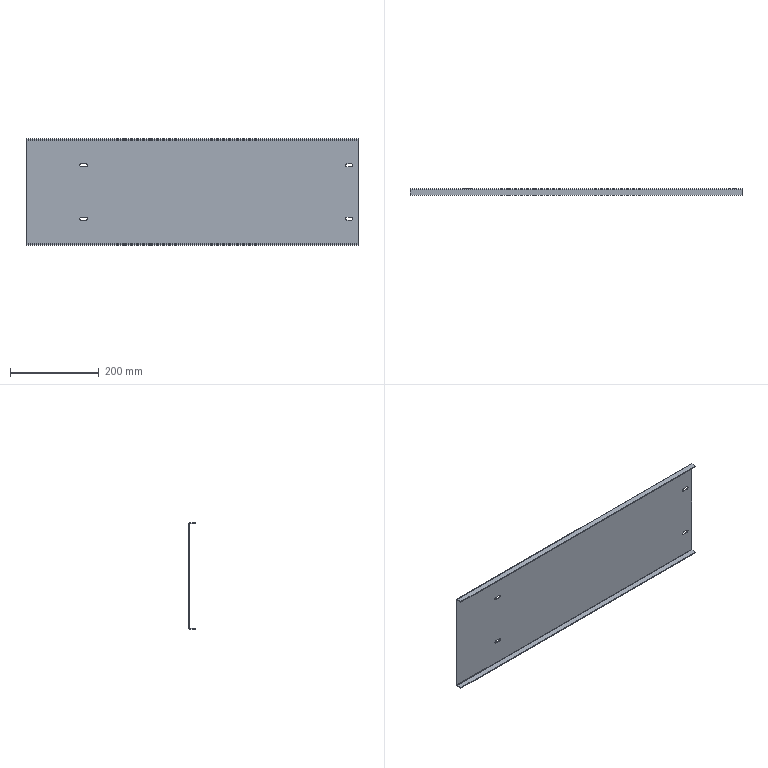Part | STEP file | PN_0026_cover plate | 1 solid | 30 faces | box 750 x 15 x 240 mm | volume 395896 mm3 | plane 18 | cylinder 12 | commonest cylinder face diameters 7 x8 1.473 x2 5.473 x2